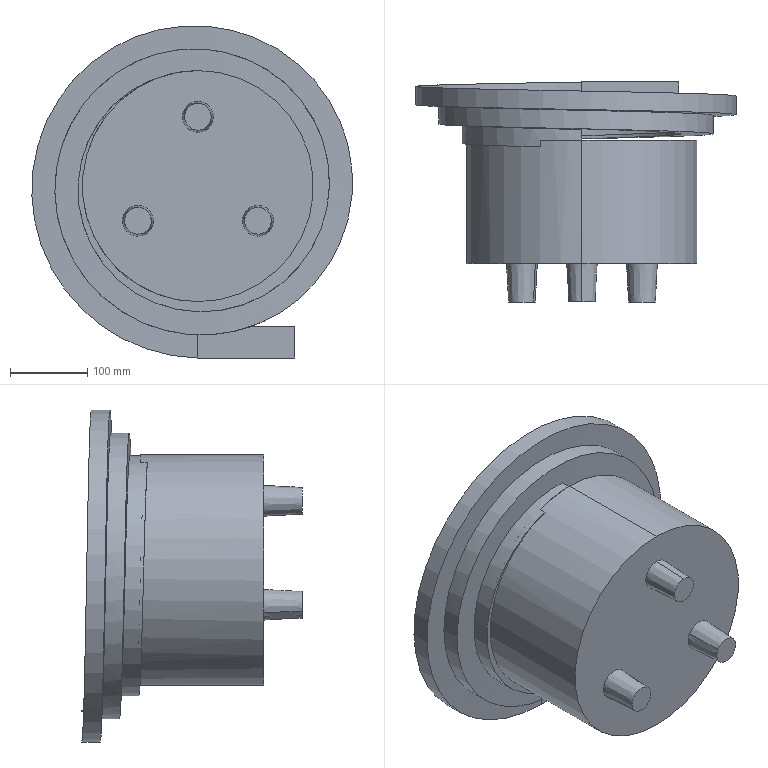Part | STEP file | Vibratory bowl feeder | 1 solid | 32 faces | box 416.592 x 286.08 x 431.538 mm | volume 12004626 mm3 | plane 16 | spline 7 | cone 6 | cylinder 3 | commonest cylinder face diameters 300 x3